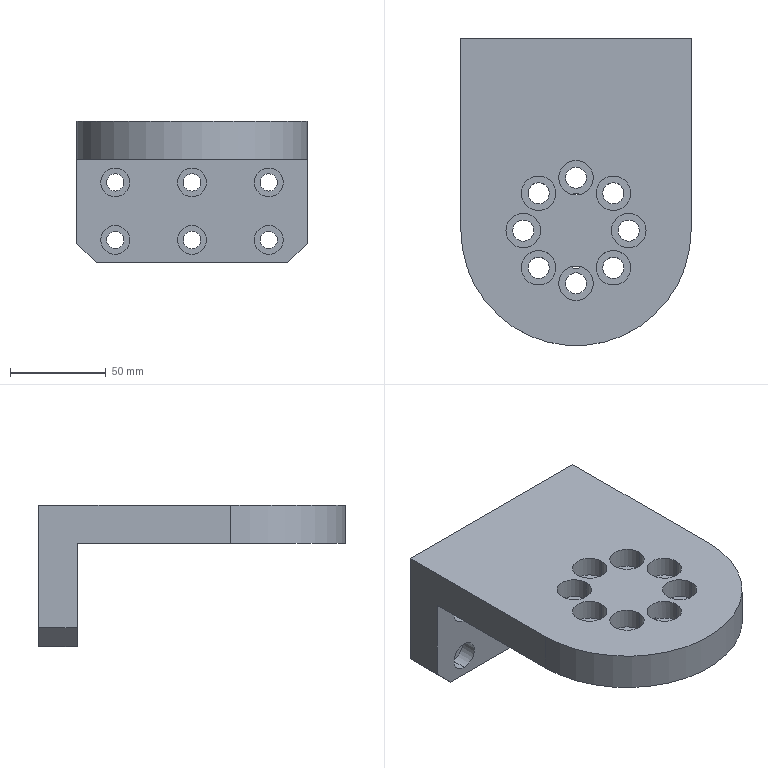Part | SolidWorks | features HoleWzd 4, Chamfer 1, Extrusion 1, ICE 1 | 1 solid | 92 faces | box 120 x 160 x 74 mm | volume 438042 mm3 | cylinder 61 | plane 27 | cone 4 | commonest cylinder face diameters 11 x16 18 x16 9 x12 15 x12 5 x4 120 x1